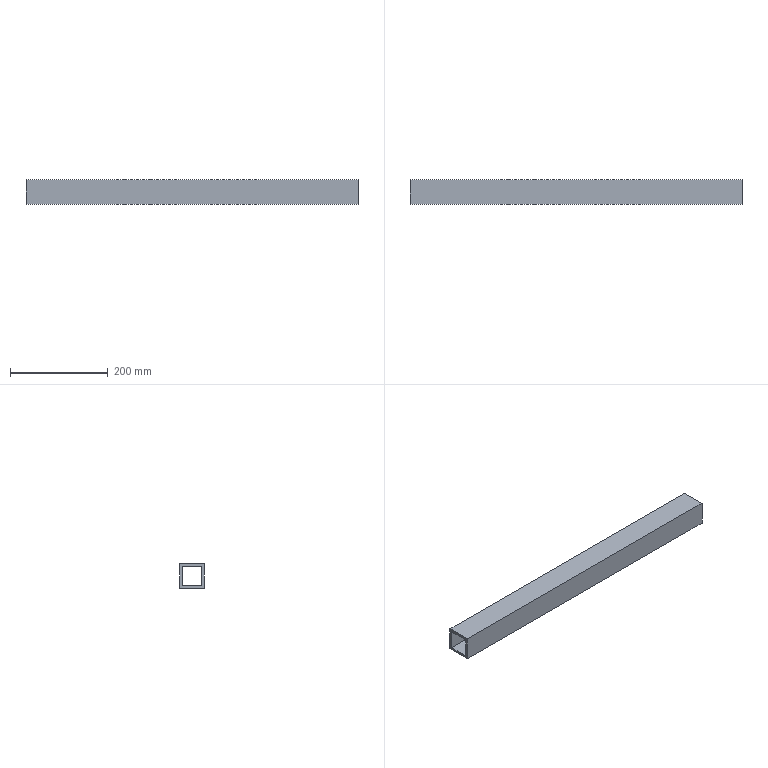Part | NX | features solid 2 | 1 solid | 10 faces | box 680 x 50 x 50 mm | volume 612000 mm3 | plane 10
STEP:
#1=CARTESIAN_POINT('',(-1060.,45.,-525.));
#2=VERTEX_POINT('',#1);
#3=CARTESIAN_POINT('',(-1060.,5.,-525.));
#4=VERTEX_POINT('',#3);
#5=CARTESIAN_POINT('',(-1060.,0.,-525.));
#6=DIRECTION('',(0.,-1.,0.));
#7=VECTOR('',#6,1000.);
#8=LINE('',#5,#7);
#9=EDGE_CURVE('',#2,#4,#8,.T.);
#10=ORIENTED_EDGE('',*,*,#9,.F.);
#11=CARTESIAN_POINT('',(-1060.,45.,-485.));
#12=VERTEX_POINT('',#11);
#13=CARTESIAN_POINT('',(-1060.,45.,-530.));
#14=DIRECTION('',(0.,0.,-1.));
#15=VECTOR('',#14,1000.);
#16=LINE('',#13,#15);
#17=EDGE_CURVE('',#12,#2,#16,.T.);
#18=ORIENTED_EDGE('',*,*,#17,.F.);
#19=CARTESIAN_POINT('',(-1060.,5.,-485.));
#20=VERTEX_POINT('',#19);
#21=CARTESIAN_POINT('',(-1060.,0.,-485.));
#22=DIRECTION('',(0.,1.,0.));
#23=VECTOR('',#22,1000.);
#24=LINE('',#21,#23);
#25=EDGE_CURVE('',#20,#12,#24,.T.);
#26=ORIENTED_EDGE('',*,*,#25,.F.);
#27=CARTESIAN_POINT('',(-1060.,5.,-530.));
#28=DIRECTION('',(0.,0.,1.));
#29=VECTOR('',#28,1000.);
#30=LINE('',#27,#29);
#31=EDGE_CURVE('',#4,#20,#30,.T.);
#32=ORIENTED_EDGE('',*,*,#31,.F.);
#33=EDGE_LOOP('',(#10,#18,#26,#32));
#34=FACE_BOUND('',#33,.T.);
#35=CARTESIAN_POINT('',(-1060.,0.,-480.));
#36=VERTEX_POINT('',#35);
#37=CARTESIAN_POINT('',(-1060.,50.,-480.));
#38=VERTEX_POINT('',#37);
#39=CARTESIAN_POINT('',(-1060.,0.,-480.));
#40=DIRECTION('',(0.,1.,0.));
#41=VECTOR('',#40,1000.);
#42=LINE('',#39,#41);
#43=EDGE_CURVE('',#36,#38,#42,.T.);
#44=ORIENTED_EDGE('',*,*,#43,.T.);
#45=CARTESIAN_POINT('',(-1060.,50.,-530.));
#46=VERTEX_POINT('',#45);
#47=CARTESIAN_POINT('',(-1060.,50.,-530.));
#48=DIRECTION('',(0.,0.,-1.));
#49=VECTOR('',#48,1000.);
#50=LINE('',#47,#49);
#51=EDGE_CURVE('',#38,#46,#50,.T.);
#52=ORIENTED_EDGE('',*,*,#51,.T.);
#53=CARTESIAN_POINT('',(-1060.,0.,-530.));
#54=VERTEX_POINT('',#53);
#55=CARTESIAN_POINT('',(-1060.,0.,-530.));
#56=DIRECTION('',(0.,-1.,0.));
#57=VECTOR('',#56,1000.);
#58=LINE('',#55,#57);
#59=EDGE_CURVE('',#46,#54,#58,.T.);
#60=ORIENTED_EDGE('',*,*,#59,.T.);
#61=CARTESIAN_POINT('',(-1060.,0.,-530.));
#62=DIRECTION('',(0.,0.,1.));
#63=VECTOR('',#62,1000.);
#64=LINE('',#61,#63);
#65=EDGE_CURVE('',#54,#36,#64,.T.);
#66=ORIENTED_EDGE('',*,*,#65,.T.);
#67=EDGE_LOOP('',(#44,#52,#60,#66));
#68=FACE_BOUND('',#67,.T.);
#69=CARTESIAN_POINT('',(-1060.,0.,-530.));
#70=DIRECTION('',(1.,0.,0.));
#71=DIRECTION('',(0.,-1.,0.));
#72=AXIS2_PLACEMENT_3D('',#69,#70,#71);
#73=PLANE('',#72);
#74=ADVANCED_FACE('',(#34,#68),#73,.F.);
#75=CARTESIAN_POINT('',(-380.,0.,-530.));
#76=VERTEX_POINT('',#75);
#77=CARTESIAN_POINT('',(-1060.,0.,-530.));
#78=DIRECTION('',(1.,0.,0.));
#79=VECTOR('',#78,1000.);
#80=LINE('',#77,#79);
#81=EDGE_CURVE('',#54,#76,#80,.T.);
#82=ORIENTED_EDGE('',*,*,#81,.T.);
#83=CARTESIAN_POINT('',(-380.,0.,-480.));
#84=VERTEX_POINT('',#83);
#85=CARTESIAN_POINT('',(-380.,0.,-530.));
#86=DIRECTION('',(0.,0.,-1.));
#87=VECTOR('',#86,1000.);
#88=LINE('',#85,#87);
#89=EDGE_CURVE('',#84,#76,#88,.T.);
#90=ORIENTED_EDGE('',*,*,#89,.F.);
#91=CARTESIAN_POINT('',(-1060.,0.,-480.));
#92=DIRECTION('',(-1.,0.,0.));
#93=VECTOR('',#92,1000.);
#94=LINE('',#91,#93);
#95=EDGE_CURVE('',#84,#36,#94,.T.);
#96=ORIENTED_EDGE('',*,*,#95,.T.);
#97=ORIENTED_EDGE('',*,*,#65,.F.);
#98=EDGE_LOOP('',(#82,#90,#96,#97));
#99=FACE_BOUND('',#98,.T.);
#100=CARTESIAN_POINT('',(-1060.,0.,-530.));
#101=DIRECTION('',(0.,1.,0.));
#102=DIRECTION('',(1.,0.,0.));
#103=AXIS2_PLACEMENT_3D('',#100,#101,#102);
#104=PLANE('',#103);
#105=ADVANCED_FACE('',(#99),#104,.F.);
#106=CARTESIAN_POINT('',(-380.,50.,-530.));
#107=VERTEX_POINT('',#106);
#108=CARTESIAN_POINT('',(-1060.,50.,-530.));
#109=DIRECTION('',(1.,0.,0.));
#110=VECTOR('',#109,1000.);
#111=LINE('',#108,#110);
#112=EDGE_CURVE('',#46,#107,#111,.T.);
#113=ORIENTED_EDGE('',*,*,#112,.T.);
#114=CARTESIAN_POINT('',(-380.,0.,-530.));
#115=DIRECTION('',(0.,1.,0.));
#116=VECTOR('',#115,1000.);
#117=LINE('',#114,#116);
#118=EDGE_CURVE('',#76,#107,#117,.T.);
#119=ORIENTED_EDGE('',*,*,#118,.F.);
#120=ORIENTED_EDGE('',*,*,#81,.F.);
#121=ORIENTED_EDGE('',*,*,#59,.F.);
#122=EDGE_LOOP('',(#113,#119,#120,#121));
#123=FACE_BOUND('',#122,.T.);
#124=CARTESIAN_POINT('',(-1060.,0.,-530.));
#125=DIRECTION('',(0.,0.,1.));
#126=DIRECTION('',(0.,-1.,0.));
#127=AXIS2_PLACEMENT_3D('',#124,#125,#126);
#128=PLANE('',#127);
#129=ADVANCED_FACE('',(#123),#128,.F.);
#130=CARTESIAN_POINT('',(-380.,50.,-480.));
#131=VERTEX_POINT('',#130);
#132=CARTESIAN_POINT('',(-1060.,50.,-480.));
#133=DIRECTION('',(1.,0.,0.));
#134=VECTOR('',#133,1000.);
#135=LINE('',#132,#134);
#136=EDGE_CURVE('',#38,#131,#135,.T.);
#137=ORIENTED_EDGE('',*,*,#136,.T.);
#138=CARTESIAN_POINT('',(-380.,50.,-480.));
#139=DIRECTION('',(0.,0.,1.));
#140=VECTOR('',#139,1000.);
#141=LINE('',#138,#140);
#142=EDGE_CURVE('',#107,#131,#141,.T.);
#143=ORIENTED_EDGE('',*,*,#142,.F.);
#144=ORIENTED_EDGE('',*,*,#112,.F.);
#145=ORIENTED_EDGE('',*,*,#51,.F.);
#146=EDGE_LOOP('',(#137,#143,#144,#145));
#147=FACE_BOUND('',#146,.T.);
#148=CARTESIAN_POINT('',(-1060.,50.,-480.));
#149=DIRECTION('',(0.,-1.,0.));
#150=DIRECTION('',(-1.,0.,0.));
#151=AXIS2_PLACEMENT_3D('',#148,#149,#150);
#152=PLANE('',#151);
#153=ADVANCED_FACE('',(#147),#152,.F.);
#154=ORIENTED_EDGE('',*,*,#95,.F.);
#155=CARTESIAN_POINT('',(-380.,0.,-480.));
#156=DIRECTION('',(0.,-1.,0.));
#157=VECTOR('',#156,1000.);
#158=LINE('',#155,#157);
#159=EDGE_CURVE('',#131,#84,#158,.T.);
#160=ORIENTED_EDGE('',*,*,#159,.F.);
#161=ORIENTED_EDGE('',*,*,#136,.F.);
#162=ORIENTED_EDGE('',*,*,#43,.F.);
#163=EDGE_LOOP('',(#154,#160,#161,#162));
#164=FACE_BOUND('',#163,.T.);
#165=CARTESIAN_POINT('',(-420.,0.,-480.));
#166=DIRECTION('',(0.,0.,-1.));
#167=DIRECTION('',(-1.,0.,0.));
#168=AXIS2_PLACEMENT_3D('',#165,#166,#167);
#169=PLANE('',#168);
#170=ADVANCED_FACE('',(#164),#169,.F.);
#171=CARTESIAN_POINT('',(-380.,45.,-525.));
#172=VERTEX_POINT('',#171);
#173=CARTESIAN_POINT('',(-380.,5.,-525.));
#174=VERTEX_POINT('',#173);
#175=CARTESIAN_POINT('',(-380.,0.,-525.));
#176=DIRECTION('',(0.,-1.,0.));
#177=VECTOR('',#176,1000.);
#178=LINE('',#175,#177);
#179=EDGE_CURVE('',#172,#174,#178,.T.);
#180=ORIENTED_EDGE('',*,*,#179,.F.);
#181=CARTESIAN_POINT('',(-1060.,45.,-525.));
#182=DIRECTION('',(1.,0.,0.));
#183=VECTOR('',#182,1000.);
#184=LINE('',#181,#183);
#185=EDGE_CURVE('',#2,#172,#184,.T.);
#186=ORIENTED_EDGE('',*,*,#185,.F.);
#187=ORIENTED_EDGE('',*,*,#9,.T.);
#188=CARTESIAN_POINT('',(-1060.,5.,-525.));
#189=DIRECTION('',(-1.,0.,0.));
#190=VECTOR('',#189,1000.);
#191=LINE('',#188,#190);
#192=EDGE_CURVE('',#174,#4,#191,.T.);
#193=ORIENTED_EDGE('',*,*,#192,.F.);
#194=EDGE_LOOP('',(#180,#186,#187,#193));
#195=FACE_BOUND('',#194,.T.);
#196=CARTESIAN_POINT('',(-1060.,45.,-525.));
#197=DIRECTION('',(0.,0.,1.));
#198=DIRECTION('',(0.,-1.,0.));
#199=AXIS2_PLACEMENT_3D('',#196,#197,#198);
#200=PLANE('',#199);
#201=ADVANCED_FACE('',(#195),#200,.T.);
#202=CARTESIAN_POINT('',(-380.,5.,-485.));
#203=VERTEX_POINT('',#202);
#204=CARTESIAN_POINT('',(-380.,5.,-530.));
#205=DIRECTION('',(0.,0.,1.));
#206=VECTOR('',#205,1000.);
#207=LINE('',#204,#206);
#208=EDGE_CURVE('',#174,#203,#207,.T.);
#209=ORIENTED_EDGE('',*,*,#208,.F.);
#210=ORIENTED_EDGE('',*,*,#192,.T.);
#211=ORIENTED_EDGE('',*,*,#31,.T.);
#212=CARTESIAN_POINT('',(-420.,5.,-485.));
#213=DIRECTION('',(-1.,0.,0.));
#214=VECTOR('',#213,1000.);
#215=LINE('',#212,#214);
#216=EDGE_CURVE('',#203,#20,#215,.T.);
#217=ORIENTED_EDGE('',*,*,#216,.F.);
#218=EDGE_LOOP('',(#209,#210,#211,#217));
#219=FACE_BOUND('',#218,.T.);
#220=CARTESIAN_POINT('',(-420.,5.,-525.));
#221=DIRECTION('',(0.,1.,0.));
#222=DIRECTION('',(1.,0.,0.));
#223=AXIS2_PLACEMENT_3D('',#220,#221,#222);
#224=PLANE('',#223);
#225=ADVANCED_FACE('',(#219),#224,.T.);
#226=CARTESIAN_POINT('',(-380.,45.,-485.));
#227=VERTEX_POINT('',#226);
#228=CARTESIAN_POINT('',(-380.,0.,-485.));
#229=DIRECTION('',(0.,1.,0.));
#230=VECTOR('',#229,1000.);
#231=LINE('',#228,#230);
#232=EDGE_CURVE('',#203,#227,#231,.T.);
#233=ORIENTED_EDGE('',*,*,#232,.F.);
#234=ORIENTED_EDGE('',*,*,#216,.T.);
#235=ORIENTED_EDGE('',*,*,#25,.T.);
#236=CARTESIAN_POINT('',(-420.,45.,-485.));
#237=DIRECTION('',(-1.,0.,0.));
#238=VECTOR('',#237,1000.);
#239=LINE('',#236,#238);
#240=EDGE_CURVE('',#227,#12,#239,.T.);
#241=ORIENTED_EDGE('',*,*,#240,.F.);
#242=EDGE_LOOP('',(#233,#234,#235,#241));
#243=FACE_BOUND('',#242,.T.);
#244=CARTESIAN_POINT('',(-420.,5.,-485.));
#245=DIRECTION('',(0.,0.,-1.));
#246=DIRECTION('',(-1.,0.,0.));
#247=AXIS2_PLACEMENT_3D('',#244,#245,#246);
#248=PLANE('',#247);
#249=ADVANCED_FACE('',(#243),#248,.T.);
#250=CARTESIAN_POINT('',(-380.,45.,-530.));
#251=DIRECTION('',(0.,0.,-1.));
#252=VECTOR('',#251,1000.);
#253=LINE('',#250,#252);
#254=EDGE_CURVE('',#227,#172,#253,.T.);
#255=ORIENTED_EDGE('',*,*,#254,.F.);
#256=ORIENTED_EDGE('',*,*,#240,.T.);
#257=ORIENTED_EDGE('',*,*,#17,.T.);
#258=ORIENTED_EDGE('',*,*,#185,.T.);
#259=EDGE_LOOP('',(#255,#256,#257,#258));
#260=FACE_BOUND('',#259,.T.);
#261=CARTESIAN_POINT('',(-1060.,45.,-485.));
#262=DIRECTION('',(0.,-1.,0.));
#263=DIRECTION('',(-1.,0.,0.));
#264=AXIS2_PLACEMENT_3D('',#261,#262,#263);
#265=PLANE('',#264);
#266=ADVANCED_FACE('',(#260),#265,.T.);
#267=ORIENTED_EDGE('',*,*,#232,.T.);
#268=ORIENTED_EDGE('',*,*,#254,.T.);
#269=ORIENTED_EDGE('',*,*,#179,.T.);
#270=ORIENTED_EDGE('',*,*,#208,.T.);
#271=EDGE_LOOP('',(#267,#268,#269,#270));
#272=FACE_BOUND('',#271,.T.);
#273=ORIENTED_EDGE('',*,*,#142,.T.);
#274=ORIENTED_EDGE('',*,*,#159,.T.);
#275=ORIENTED_EDGE('',*,*,#89,.T.);
#276=ORIENTED_EDGE('',*,*,#118,.T.);
#277=EDGE_LOOP('',(#273,#274,#275,#276));
#278=FACE_BOUND('',#277,.T.);
#279=CARTESIAN_POINT('',(-380.,0.,-530.));
#280=DIRECTION('',(1.,0.,0.));
#281=DIRECTION('',(0.,-1.,0.));
#282=AXIS2_PLACEMENT_3D('',#279,#280,#281);
#283=PLANE('',#282);
#284=ADVANCED_FACE('',(#272,#278),#283,.T.);
#285=CLOSED_SHELL('',(#74,#105,#129,#153,#170,#201,#225,#249,#266,#284));
#286=MANIFOLD_SOLID_BREP('',#285);
#287=(LENGTH_UNIT()NAMED_UNIT(*)SI_UNIT(.MILLI.,.METRE.));
#288=UNCERTAINTY_MEASURE_WITH_UNIT(LENGTH_MEASURE(0.00001),#287,'','');
#289=(NAMED_UNIT(*)PLANE_ANGLE_UNIT()SI_UNIT($,.RADIAN.));
#290=(NAMED_UNIT(*)SI_UNIT($,.STERADIAN.)SOLID_ANGLE_UNIT());
#291=(GEOMETRIC_REPRESENTATION_CONTEXT(3)GLOBAL_UNCERTAINTY_ASSIGNED_CONTEXT((#288))GLOBAL_UNIT_ASSIGNED_CONTEXT((#287,#289,#290))REPRESENTATION_CONTEXT('',''));
#292=ADVANCED_BREP_SHAPE_REPRESENTATION('',(#286),#291);